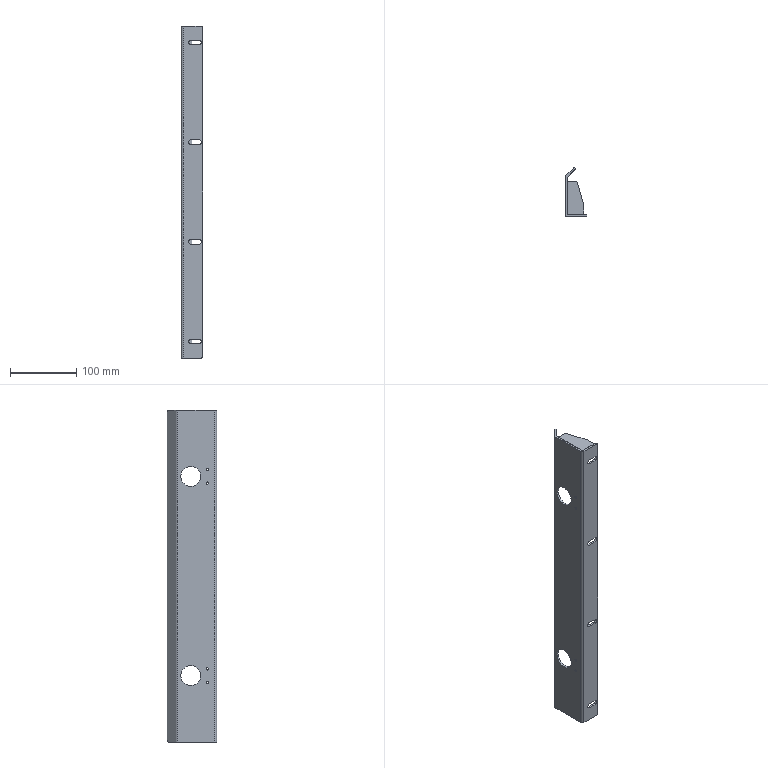Part | STEP file | KF-2212-070-005 | 4 solids | 75 faces | box 33 x 74.142 x 500 mm | volume 165565 mm3 | plane 47 | cylinder 28 | commonest cylinder face diameters 7 x10 3.3 x8 5 x4 30 x4 1 x2